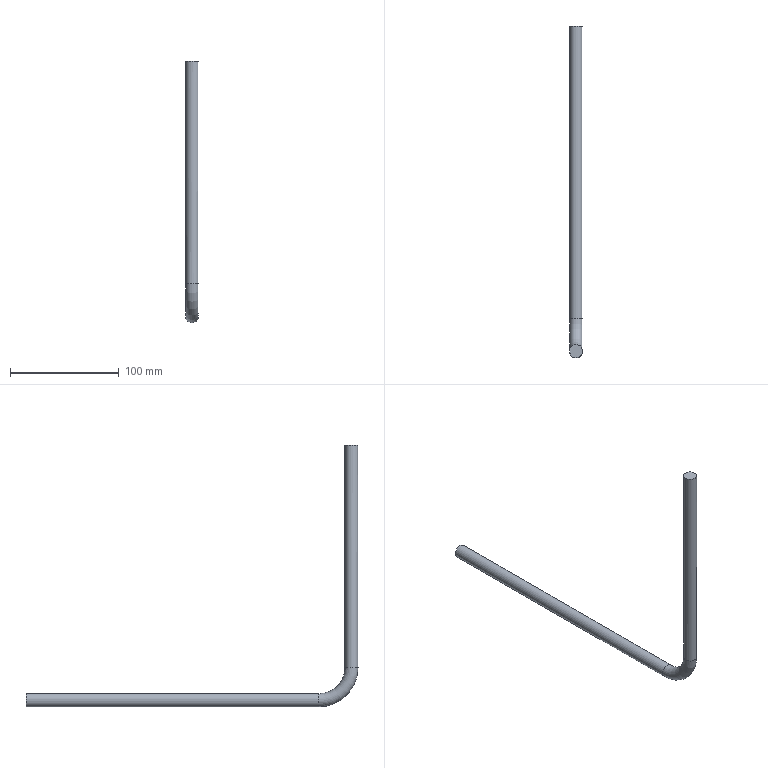Part | NX | features solid 2 | 1 solid | 5 faces | box 12 x 306 x 241 mm | volume 59051 mm3 | plane 2 | cylinder 2 | torus 1 | commonest cylinder face diameters 12 x2
STEP:
#1=CARTESIAN_POINT('',(161.,75.,-250.));
#2=VERTEX_POINT('',#1);
#3=CARTESIAN_POINT('',(155.,75.,-250.));
#4=DIRECTION('',(0.,0.,1.));
#5=DIRECTION('',(1.,0.,0.));
#6=AXIS2_PLACEMENT_3D('',#3,#4,#5);
#7=CIRCLE('',#6,6.);
#8=EDGE_CURVE('',#2,#2,#7,.F.);
#9=ORIENTED_EDGE('',*,*,#8,.F.);
#10=EDGE_LOOP('',(#9));
#11=FACE_BOUND('',#10,.T.);
#12=CARTESIAN_POINT('',(0.,-30.,-250.));
#13=DIRECTION('',(0.,0.,1.));
#14=DIRECTION('',(1.,0.,0.));
#15=AXIS2_PLACEMENT_3D('',#12,#13,#14);
#16=PLANE('',#15);
#17=ADVANCED_FACE('',(#11),#16,.T.);
#18=CARTESIAN_POINT('',(155.,81.,-455.));
#19=VERTEX_POINT('',#18);
#20=CARTESIAN_POINT('',(155.,75.,-455.));
#21=DIRECTION('',(0.,0.,-1.));
#22=DIRECTION('',(0.,1.,0.));
#23=AXIS2_PLACEMENT_3D('',#20,#21,#22);
#24=CIRCLE('',#23,6.);
#25=EDGE_CURVE('',#19,#19,#24,.T.);
#26=ORIENTED_EDGE('',*,*,#25,.F.);
#27=EDGE_LOOP('',(#26));
#28=FACE_BOUND('',#27,.T.);
#29=ORIENTED_EDGE('',*,*,#8,.T.);
#30=EDGE_LOOP('',(#29));
#31=FACE_BOUND('',#30,.T.);
#32=CARTESIAN_POINT('',(155.,75.,-197.5));
#33=DIRECTION('',(0.,0.,-1.));
#34=DIRECTION('',(-1.,0.,0.));
#35=AXIS2_PLACEMENT_3D('',#32,#33,#34);
#36=CYLINDRICAL_SURFACE('',#35,6.);
#37=ADVANCED_FACE('',(#28,#31),#36,.T.);
#38=CARTESIAN_POINT('',(155.,105.,-479.));
#39=VERTEX_POINT('',#38);
#40=CARTESIAN_POINT('',(155.,105.,-485.));
#41=DIRECTION('',(0.,1.,0.));
#42=DIRECTION('',(0.,0.,1.));
#43=AXIS2_PLACEMENT_3D('',#40,#41,#42);
#44=CIRCLE('',#43,6.);
#45=EDGE_CURVE('',#39,#39,#44,.T.);
#46=ORIENTED_EDGE('',*,*,#45,.T.);
#47=EDGE_LOOP('',(#46));
#48=FACE_BOUND('',#47,.T.);
#49=CARTESIAN_POINT('',(155.,375.,-479.));
#50=VERTEX_POINT('',#49);
#51=CARTESIAN_POINT('',(155.,375.,-485.));
#52=DIRECTION('',(0.,1.,0.));
#53=DIRECTION('',(0.,0.,1.));
#54=AXIS2_PLACEMENT_3D('',#51,#52,#53);
#55=CIRCLE('',#54,6.);
#56=EDGE_CURVE('',#50,#50,#55,.T.);
#57=ORIENTED_EDGE('',*,*,#56,.F.);
#58=EDGE_LOOP('',(#57));
#59=FACE_BOUND('',#58,.T.);
#60=CARTESIAN_POINT('',(155.,105.,-485.));
#61=DIRECTION('',(0.,1.,0.));
#62=DIRECTION('',(-1.,0.,0.));
#63=AXIS2_PLACEMENT_3D('',#60,#61,#62);
#64=CYLINDRICAL_SURFACE('',#63,6.);
#65=ADVANCED_FACE('',(#48,#59),#64,.T.);
#66=ORIENTED_EDGE('',*,*,#25,.T.);
#67=EDGE_LOOP('',(#66));
#68=FACE_BOUND('',#67,.T.);
#69=ORIENTED_EDGE('',*,*,#45,.F.);
#70=EDGE_LOOP('',(#69));
#71=FACE_BOUND('',#70,.T.);
#72=CARTESIAN_POINT('',(155.,105.,-455.));
#73=DIRECTION('',(1.,0.,0.));
#74=DIRECTION('',(0.,0.,-1.));
#75=AXIS2_PLACEMENT_3D('',#72,#73,#74);
#76=TOROIDAL_SURFACE('',#75,30.,6.);
#77=ADVANCED_FACE('',(#68,#71),#76,.T.);
#78=ORIENTED_EDGE('',*,*,#56,.T.);
#79=EDGE_LOOP('',(#78));
#80=FACE_BOUND('',#79,.T.);
#81=CARTESIAN_POINT('',(155.,375.,-485.));
#82=DIRECTION('',(0.,1.,0.));
#83=DIRECTION('',(0.,0.,1.));
#84=AXIS2_PLACEMENT_3D('',#81,#82,#83);
#85=PLANE('',#84);
#86=ADVANCED_FACE('',(#80),#85,.T.);
#87=CLOSED_SHELL('',(#17,#37,#65,#77,#86));
#88=MANIFOLD_SOLID_BREP('',#87);
#89=(LENGTH_UNIT()NAMED_UNIT(*)SI_UNIT(.MILLI.,.METRE.));
#90=UNCERTAINTY_MEASURE_WITH_UNIT(LENGTH_MEASURE(0.00001),#89,'','');
#91=(NAMED_UNIT(*)PLANE_ANGLE_UNIT()SI_UNIT($,.RADIAN.));
#92=(NAMED_UNIT(*)SI_UNIT($,.STERADIAN.)SOLID_ANGLE_UNIT());
#93=(GEOMETRIC_REPRESENTATION_CONTEXT(3)GLOBAL_UNCERTAINTY_ASSIGNED_CONTEXT((#90))GLOBAL_UNIT_ASSIGNED_CONTEXT((#89,#91,#92))REPRESENTATION_CONTEXT('',''));
#94=ADVANCED_BREP_SHAPE_REPRESENTATION('',(#88),#93);